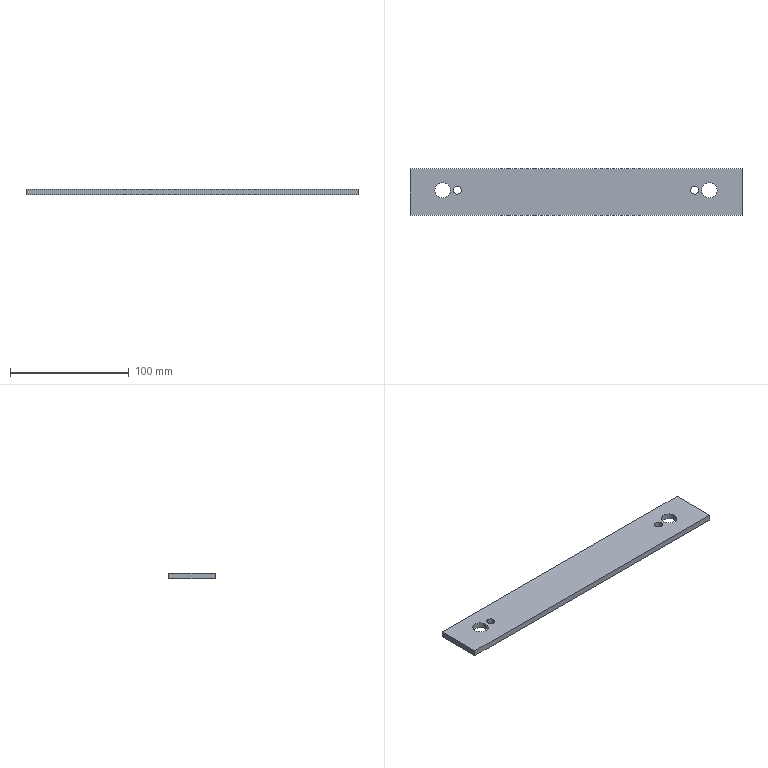Part | STEP file | 44-02-09 Ear Forming Plate B | 1 solid | 14 faces | box 280 x 39 x 5 mm | volume 52910 mm3 | cylinder 8 | plane 6 | commonest cylinder face diameters 6.8 x4 13 x4
STEP:
#1=CARTESIAN_POINT('',(0.,0.,0.));
#2=DIRECTION('',(0.,0.,1.));
#3=DIRECTION('',(1.,0.,0.));
#4=AXIS2_PLACEMENT_3D('',#1,#2,#3);
#5=CARTESIAN_POINT('',(-96.6,0.,-2.5));
#6=VERTEX_POINT('',#5);
#7=CARTESIAN_POINT('',(-96.6,0.,2.5));
#8=VERTEX_POINT('',#7);
#9=CARTESIAN_POINT('',(-96.6,0.,2.5));
#10=DIRECTION('',(0.,0.,1.));
#11=VECTOR('',#10,1.);
#12=LINE('',#9,#11);
#13=CARTESIAN_POINT('',(-100.,0.,2.5));
#14=DIRECTION('',(0.,0.,1.));
#15=DIRECTION('',(1.,0.,0.));
#16=AXIS2_PLACEMENT_3D('',#13,#14,#15);
#17=CYLINDRICAL_SURFACE('',#16,3.4);
#18=CARTESIAN_POINT('',(6.283,0.));
#19=DIRECTION('',(0.,1.));
#20=VECTOR('',#19,1.);
#21=LINE('',#18,#20);
#22=(GEOMETRIC_REPRESENTATION_CONTEXT(2)PARAMETRIC_REPRESENTATION_CONTEXT()REPRESENTATION_CONTEXT('',''));
#23=DEFINITIONAL_REPRESENTATION('',(#21),#22);
#24=PCURVE('',#17,#23);
#25=CARTESIAN_POINT('',(-100.,0.,2.5));
#26=DIRECTION('',(0.,0.,1.));
#27=DIRECTION('',(1.,0.,0.));
#28=AXIS2_PLACEMENT_3D('',#25,#26,#27);
#29=CYLINDRICAL_SURFACE('',#28,3.4);
#30=CARTESIAN_POINT('',(0.,0.));
#31=DIRECTION('',(0.,1.));
#32=VECTOR('',#31,1.);
#33=LINE('',#30,#32);
#34=(GEOMETRIC_REPRESENTATION_CONTEXT(2)PARAMETRIC_REPRESENTATION_CONTEXT()REPRESENTATION_CONTEXT('',''));
#35=DEFINITIONAL_REPRESENTATION('',(#33),#34);
#36=PCURVE('',#29,#35);
#37=SURFACE_CURVE('',#12,(#24,#36),.PCURVE_S1.);
#38=EDGE_CURVE('',#6,#8,#37,.T.);
#39=ORIENTED_EDGE('',*,*,#38,.T.);
#40=CARTESIAN_POINT('',(-103.4,0.,2.5));
#41=VERTEX_POINT('',#40);
#42=CARTESIAN_POINT('',(-100.,0.,2.5));
#43=DIRECTION('',(0.,0.,1.));
#44=DIRECTION('',(1.,0.,0.));
#45=AXIS2_PLACEMENT_3D('',#42,#43,#44);
#46=CIRCLE('',#45,3.4);
#47=CARTESIAN_POINT('',(0.,0.));
#48=DIRECTION('',(1.,0.));
#49=VECTOR('',#48,1.);
#50=LINE('',#47,#49);
#51=(GEOMETRIC_REPRESENTATION_CONTEXT(2)PARAMETRIC_REPRESENTATION_CONTEXT()REPRESENTATION_CONTEXT('',''));
#52=DEFINITIONAL_REPRESENTATION('',(#50),#51);
#53=PCURVE('',#17,#52);
#54=CARTESIAN_POINT('',(140.,-18.,2.5));
#55=DIRECTION('',(0.,0.,1.));
#56=DIRECTION('',(1.,0.,0.));
#57=AXIS2_PLACEMENT_3D('',#54,#55,#56);
#58=PLANE('',#57);
#59=CARTESIAN_POINT('',(-240.,18.));
#60=DIRECTION('',(1.,0.));
#61=AXIS2_PLACEMENT_2D('',#59,#60);
#62=CIRCLE('',#61,3.4);
#63=(GEOMETRIC_REPRESENTATION_CONTEXT(2)PARAMETRIC_REPRESENTATION_CONTEXT()REPRESENTATION_CONTEXT('',''));
#64=DEFINITIONAL_REPRESENTATION('',(#62),#63);
#65=PCURVE('',#58,#64);
#66=SURFACE_CURVE('',#46,(#53,#65),.PCURVE_S1.);
#67=EDGE_CURVE('',#41,#8,#66,.T.);
#68=ORIENTED_EDGE('',*,*,#67,.F.);
#69=CARTESIAN_POINT('',(-103.4,0.,-2.5));
#70=VERTEX_POINT('',#69);
#71=CARTESIAN_POINT('',(-103.4,0.,2.5));
#72=DIRECTION('',(0.,0.,1.));
#73=VECTOR('',#72,1.);
#74=LINE('',#71,#73);
#75=CARTESIAN_POINT('',(3.142,0.));
#76=DIRECTION('',(0.,1.));
#77=VECTOR('',#76,1.);
#78=LINE('',#75,#77);
#79=(GEOMETRIC_REPRESENTATION_CONTEXT(2)PARAMETRIC_REPRESENTATION_CONTEXT()REPRESENTATION_CONTEXT('',''));
#80=DEFINITIONAL_REPRESENTATION('',(#78),#79);
#81=PCURVE('',#17,#80);
#82=CARTESIAN_POINT('',(3.142,0.));
#83=DIRECTION('',(0.,1.));
#84=VECTOR('',#83,1.);
#85=LINE('',#82,#84);
#86=(GEOMETRIC_REPRESENTATION_CONTEXT(2)PARAMETRIC_REPRESENTATION_CONTEXT()REPRESENTATION_CONTEXT('',''));
#87=DEFINITIONAL_REPRESENTATION('',(#85),#86);
#88=PCURVE('',#29,#87);
#89=SURFACE_CURVE('',#74,(#81,#88),.PCURVE_S1.);
#90=EDGE_CURVE('',#70,#41,#89,.T.);
#91=ORIENTED_EDGE('',*,*,#90,.F.);
#92=CARTESIAN_POINT('',(-100.,0.,-2.5));
#93=DIRECTION('',(0.,0.,1.));
#94=DIRECTION('',(1.,0.,0.));
#95=AXIS2_PLACEMENT_3D('',#92,#93,#94);
#96=CIRCLE('',#95,3.4);
#97=CARTESIAN_POINT('',(0.,-5.));
#98=DIRECTION('',(1.,0.));
#99=VECTOR('',#98,1.);
#100=LINE('',#97,#99);
#101=(GEOMETRIC_REPRESENTATION_CONTEXT(2)PARAMETRIC_REPRESENTATION_CONTEXT()REPRESENTATION_CONTEXT('',''));
#102=DEFINITIONAL_REPRESENTATION('',(#100),#101);
#103=PCURVE('',#17,#102);
#104=CARTESIAN_POINT('',(140.,-18.,-2.5));
#105=DIRECTION('',(0.,0.,1.));
#106=DIRECTION('',(1.,0.,0.));
#107=AXIS2_PLACEMENT_3D('',#104,#105,#106);
#108=PLANE('',#107);
#109=CARTESIAN_POINT('',(-240.,18.));
#110=DIRECTION('',(1.,0.));
#111=AXIS2_PLACEMENT_2D('',#109,#110);
#112=CIRCLE('',#111,3.4);
#113=(GEOMETRIC_REPRESENTATION_CONTEXT(2)PARAMETRIC_REPRESENTATION_CONTEXT()REPRESENTATION_CONTEXT('',''));
#114=DEFINITIONAL_REPRESENTATION('',(#112),#113);
#115=PCURVE('',#108,#114);
#116=SURFACE_CURVE('',#96,(#103,#115),.PCURVE_S1.);
#117=EDGE_CURVE('',#70,#6,#116,.T.);
#118=ORIENTED_EDGE('',*,*,#117,.T.);
#119=EDGE_LOOP('',(#39,#68,#91,#118));
#120=FACE_BOUND('',#119,.F.);
#121=ADVANCED_FACE('',(#120),#17,.F.);
#122=CARTESIAN_POINT('',(103.4,0.,-2.5));
#123=VERTEX_POINT('',#122);
#124=CARTESIAN_POINT('',(103.4,0.,2.5));
#125=VERTEX_POINT('',#124);
#126=CARTESIAN_POINT('',(103.4,0.,2.5));
#127=DIRECTION('',(0.,0.,1.));
#128=VECTOR('',#127,1.);
#129=LINE('',#126,#128);
#130=CARTESIAN_POINT('',(100.,0.,2.5));
#131=DIRECTION('',(0.,0.,1.));
#132=DIRECTION('',(1.,0.,0.));
#133=AXIS2_PLACEMENT_3D('',#130,#131,#132);
#134=CYLINDRICAL_SURFACE('',#133,3.4);
#135=CARTESIAN_POINT('',(6.283,0.));
#136=DIRECTION('',(0.,1.));
#137=VECTOR('',#136,1.);
#138=LINE('',#135,#137);
#139=(GEOMETRIC_REPRESENTATION_CONTEXT(2)PARAMETRIC_REPRESENTATION_CONTEXT()REPRESENTATION_CONTEXT('',''));
#140=DEFINITIONAL_REPRESENTATION('',(#138),#139);
#141=PCURVE('',#134,#140);
#142=CARTESIAN_POINT('',(100.,0.,2.5));
#143=DIRECTION('',(0.,0.,1.));
#144=DIRECTION('',(1.,0.,0.));
#145=AXIS2_PLACEMENT_3D('',#142,#143,#144);
#146=CYLINDRICAL_SURFACE('',#145,3.4);
#147=CARTESIAN_POINT('',(0.,0.));
#148=DIRECTION('',(0.,1.));
#149=VECTOR('',#148,1.);
#150=LINE('',#147,#149);
#151=(GEOMETRIC_REPRESENTATION_CONTEXT(2)PARAMETRIC_REPRESENTATION_CONTEXT()REPRESENTATION_CONTEXT('',''));
#152=DEFINITIONAL_REPRESENTATION('',(#150),#151);
#153=PCURVE('',#146,#152);
#154=SURFACE_CURVE('',#129,(#141,#153),.PCURVE_S1.);
#155=EDGE_CURVE('',#123,#125,#154,.T.);
#156=ORIENTED_EDGE('',*,*,#155,.T.);
#157=CARTESIAN_POINT('',(96.6,0.,2.5));
#158=VERTEX_POINT('',#157);
#159=CARTESIAN_POINT('',(100.,0.,2.5));
#160=DIRECTION('',(0.,0.,1.));
#161=DIRECTION('',(1.,0.,0.));
#162=AXIS2_PLACEMENT_3D('',#159,#160,#161);
#163=CIRCLE('',#162,3.4);
#164=CARTESIAN_POINT('',(0.,0.));
#165=DIRECTION('',(1.,0.));
#166=VECTOR('',#165,1.);
#167=LINE('',#164,#166);
#168=(GEOMETRIC_REPRESENTATION_CONTEXT(2)PARAMETRIC_REPRESENTATION_CONTEXT()REPRESENTATION_CONTEXT('',''));
#169=DEFINITIONAL_REPRESENTATION('',(#167),#168);
#170=PCURVE('',#134,#169);
#171=CARTESIAN_POINT('',(-40.,18.));
#172=DIRECTION('',(1.,0.));
#173=AXIS2_PLACEMENT_2D('',#171,#172);
#174=CIRCLE('',#173,3.4);
#175=(GEOMETRIC_REPRESENTATION_CONTEXT(2)PARAMETRIC_REPRESENTATION_CONTEXT()REPRESENTATION_CONTEXT('',''));
#176=DEFINITIONAL_REPRESENTATION('',(#174),#175);
#177=PCURVE('',#58,#176);
#178=SURFACE_CURVE('',#163,(#170,#177),.PCURVE_S1.);
#179=EDGE_CURVE('',#158,#125,#178,.T.);
#180=ORIENTED_EDGE('',*,*,#179,.F.);
#181=CARTESIAN_POINT('',(96.6,0.,-2.5));
#182=VERTEX_POINT('',#181);
#183=CARTESIAN_POINT('',(96.6,0.,2.5));
#184=DIRECTION('',(0.,0.,1.));
#185=VECTOR('',#184,1.);
#186=LINE('',#183,#185);
#187=CARTESIAN_POINT('',(3.142,0.));
#188=DIRECTION('',(0.,1.));
#189=VECTOR('',#188,1.);
#190=LINE('',#187,#189);
#191=(GEOMETRIC_REPRESENTATION_CONTEXT(2)PARAMETRIC_REPRESENTATION_CONTEXT()REPRESENTATION_CONTEXT('',''));
#192=DEFINITIONAL_REPRESENTATION('',(#190),#191);
#193=PCURVE('',#134,#192);
#194=CARTESIAN_POINT('',(3.142,0.));
#195=DIRECTION('',(0.,1.));
#196=VECTOR('',#195,1.);
#197=LINE('',#194,#196);
#198=(GEOMETRIC_REPRESENTATION_CONTEXT(2)PARAMETRIC_REPRESENTATION_CONTEXT()REPRESENTATION_CONTEXT('',''));
#199=DEFINITIONAL_REPRESENTATION('',(#197),#198);
#200=PCURVE('',#146,#199);
#201=SURFACE_CURVE('',#186,(#193,#200),.PCURVE_S1.);
#202=EDGE_CURVE('',#182,#158,#201,.T.);
#203=ORIENTED_EDGE('',*,*,#202,.F.);
#204=CARTESIAN_POINT('',(100.,0.,-2.5));
#205=DIRECTION('',(0.,0.,1.));
#206=DIRECTION('',(1.,0.,0.));
#207=AXIS2_PLACEMENT_3D('',#204,#205,#206);
#208=CIRCLE('',#207,3.4);
#209=CARTESIAN_POINT('',(0.,-5.));
#210=DIRECTION('',(1.,0.));
#211=VECTOR('',#210,1.);
#212=LINE('',#209,#211);
#213=(GEOMETRIC_REPRESENTATION_CONTEXT(2)PARAMETRIC_REPRESENTATION_CONTEXT()REPRESENTATION_CONTEXT('',''));
#214=DEFINITIONAL_REPRESENTATION('',(#212),#213);
#215=PCURVE('',#134,#214);
#216=CARTESIAN_POINT('',(-40.,18.));
#217=DIRECTION('',(1.,0.));
#218=AXIS2_PLACEMENT_2D('',#216,#217);
#219=CIRCLE('',#218,3.4);
#220=(GEOMETRIC_REPRESENTATION_CONTEXT(2)PARAMETRIC_REPRESENTATION_CONTEXT()REPRESENTATION_CONTEXT('',''));
#221=DEFINITIONAL_REPRESENTATION('',(#219),#220);
#222=PCURVE('',#108,#221);
#223=SURFACE_CURVE('',#208,(#215,#222),.PCURVE_S1.);
#224=EDGE_CURVE('',#182,#123,#223,.T.);
#225=ORIENTED_EDGE('',*,*,#224,.T.);
#226=EDGE_LOOP('',(#156,#180,#203,#225));
#227=FACE_BOUND('',#226,.F.);
#228=ADVANCED_FACE('',(#227),#134,.F.);
#229=CARTESIAN_POINT('',(119.,0.,-2.5));
#230=VERTEX_POINT('',#229);
#231=CARTESIAN_POINT('',(119.,0.,2.5));
#232=VERTEX_POINT('',#231);
#233=CARTESIAN_POINT('',(119.,0.,-2.5));
#234=DIRECTION('',(0.,0.,1.));
#235=VECTOR('',#234,1.);
#236=LINE('',#233,#235);
#237=CARTESIAN_POINT('',(112.5,0.,-2.5));
#238=DIRECTION('',(0.,0.,1.));
#239=DIRECTION('',(1.,0.,0.));
#240=AXIS2_PLACEMENT_3D('',#237,#238,#239);
#241=CYLINDRICAL_SURFACE('',#240,6.5);
#242=CARTESIAN_POINT('',(6.283,0.));
#243=DIRECTION('',(0.,1.));
#244=VECTOR('',#243,1.);
#245=LINE('',#242,#244);
#246=(GEOMETRIC_REPRESENTATION_CONTEXT(2)PARAMETRIC_REPRESENTATION_CONTEXT()REPRESENTATION_CONTEXT('',''));
#247=DEFINITIONAL_REPRESENTATION('',(#245),#246);
#248=PCURVE('',#241,#247);
#249=CARTESIAN_POINT('',(112.5,0.,-2.5));
#250=DIRECTION('',(0.,0.,1.));
#251=DIRECTION('',(1.,0.,0.));
#252=AXIS2_PLACEMENT_3D('',#249,#250,#251);
#253=CYLINDRICAL_SURFACE('',#252,6.5);
#254=CARTESIAN_POINT('',(0.,0.));
#255=DIRECTION('',(0.,1.));
#256=VECTOR('',#255,1.);
#257=LINE('',#254,#256);
#258=(GEOMETRIC_REPRESENTATION_CONTEXT(2)PARAMETRIC_REPRESENTATION_CONTEXT()REPRESENTATION_CONTEXT('',''));
#259=DEFINITIONAL_REPRESENTATION('',(#257),#258);
#260=PCURVE('',#253,#259);
#261=SURFACE_CURVE('',#236,(#248,#260),.PCURVE_S1.);
#262=EDGE_CURVE('',#230,#232,#261,.T.);
#263=ORIENTED_EDGE('',*,*,#262,.T.);
#264=CARTESIAN_POINT('',(106.,0.,2.5));
#265=VERTEX_POINT('',#264);
#266=CARTESIAN_POINT('',(112.5,0.,2.5));
#267=DIRECTION('',(0.,0.,1.));
#268=DIRECTION('',(1.,0.,0.));
#269=AXIS2_PLACEMENT_3D('',#266,#267,#268);
#270=CIRCLE('',#269,6.5);
#271=CARTESIAN_POINT('',(0.,5.));
#272=DIRECTION('',(1.,0.));
#273=VECTOR('',#272,1.);
#274=LINE('',#271,#273);
#275=(GEOMETRIC_REPRESENTATION_CONTEXT(2)PARAMETRIC_REPRESENTATION_CONTEXT()REPRESENTATION_CONTEXT('',''));
#276=DEFINITIONAL_REPRESENTATION('',(#274),#275);
#277=PCURVE('',#241,#276);
#278=CARTESIAN_POINT('',(-27.5,18.));
#279=DIRECTION('',(1.,0.));
#280=AXIS2_PLACEMENT_2D('',#278,#279);
#281=CIRCLE('',#280,6.5);
#282=(GEOMETRIC_REPRESENTATION_CONTEXT(2)PARAMETRIC_REPRESENTATION_CONTEXT()REPRESENTATION_CONTEXT('',''));
#283=DEFINITIONAL_REPRESENTATION('',(#281),#282);
#284=PCURVE('',#58,#283);
#285=SURFACE_CURVE('',#270,(#277,#284),.PCURVE_S1.);
#286=EDGE_CURVE('',#265,#232,#285,.T.);
#287=ORIENTED_EDGE('',*,*,#286,.F.);
#288=CARTESIAN_POINT('',(106.,0.,-2.5));
#289=VERTEX_POINT('',#288);
#290=CARTESIAN_POINT('',(106.,0.,-2.5));
#291=DIRECTION('',(0.,0.,1.));
#292=VECTOR('',#291,1.);
#293=LINE('',#290,#292);
#294=CARTESIAN_POINT('',(3.142,0.));
#295=DIRECTION('',(0.,1.));
#296=VECTOR('',#295,1.);
#297=LINE('',#294,#296);
#298=(GEOMETRIC_REPRESENTATION_CONTEXT(2)PARAMETRIC_REPRESENTATION_CONTEXT()REPRESENTATION_CONTEXT('',''));
#299=DEFINITIONAL_REPRESENTATION('',(#297),#298);
#300=PCURVE('',#241,#299);
#301=CARTESIAN_POINT('',(3.142,0.));
#302=DIRECTION('',(0.,1.));
#303=VECTOR('',#302,1.);
#304=LINE('',#301,#303);
#305=(GEOMETRIC_REPRESENTATION_CONTEXT(2)PARAMETRIC_REPRESENTATION_CONTEXT()REPRESENTATION_CONTEXT('',''));
#306=DEFINITIONAL_REPRESENTATION('',(#304),#305);
#307=PCURVE('',#253,#306);
#308=SURFACE_CURVE('',#293,(#300,#307),.PCURVE_S1.);
#309=EDGE_CURVE('',#289,#265,#308,.T.);
#310=ORIENTED_EDGE('',*,*,#309,.F.);
#311=CARTESIAN_POINT('',(112.5,0.,-2.5));
#312=DIRECTION('',(0.,0.,1.));
#313=DIRECTION('',(1.,0.,0.));
#314=AXIS2_PLACEMENT_3D('',#311,#312,#313);
#315=CIRCLE('',#314,6.5);
#316=CARTESIAN_POINT('',(0.,0.));
#317=DIRECTION('',(1.,0.));
#318=VECTOR('',#317,1.);
#319=LINE('',#316,#318);
#320=(GEOMETRIC_REPRESENTATION_CONTEXT(2)PARAMETRIC_REPRESENTATION_CONTEXT()REPRESENTATION_CONTEXT('',''));
#321=DEFINITIONAL_REPRESENTATION('',(#319),#320);
#322=PCURVE('',#241,#321);
#323=CARTESIAN_POINT('',(-27.5,18.));
#324=DIRECTION('',(1.,0.));
#325=AXIS2_PLACEMENT_2D('',#323,#324);
#326=CIRCLE('',#325,6.5);
#327=(GEOMETRIC_REPRESENTATION_CONTEXT(2)PARAMETRIC_REPRESENTATION_CONTEXT()REPRESENTATION_CONTEXT('',''));
#328=DEFINITIONAL_REPRESENTATION('',(#326),#327);
#329=PCURVE('',#108,#328);
#330=SURFACE_CURVE('',#315,(#322,#329),.PCURVE_S1.);
#331=EDGE_CURVE('',#289,#230,#330,.T.);
#332=ORIENTED_EDGE('',*,*,#331,.T.);
#333=EDGE_LOOP('',(#263,#287,#310,#332));
#334=FACE_BOUND('',#333,.F.);
#335=ADVANCED_FACE('',(#334),#241,.F.);
#336=CARTESIAN_POINT('',(-106.,0.,-2.5));
#337=VERTEX_POINT('',#336);
#338=CARTESIAN_POINT('',(-106.,0.,2.5));
#339=VERTEX_POINT('',#338);
#340=CARTESIAN_POINT('',(-106.,0.,-2.5));
#341=DIRECTION('',(0.,0.,1.));
#342=VECTOR('',#341,1.);
#343=LINE('',#340,#342);
#344=CARTESIAN_POINT('',(-112.5,0.,-2.5));
#345=DIRECTION('',(0.,0.,1.));
#346=DIRECTION('',(1.,0.,0.));
#347=AXIS2_PLACEMENT_3D('',#344,#345,#346);
#348=CYLINDRICAL_SURFACE('',#347,6.5);
#349=CARTESIAN_POINT('',(6.283,0.));
#350=DIRECTION('',(0.,1.));
#351=VECTOR('',#350,1.);
#352=LINE('',#349,#351);
#353=(GEOMETRIC_REPRESENTATION_CONTEXT(2)PARAMETRIC_REPRESENTATION_CONTEXT()REPRESENTATION_CONTEXT('',''));
#354=DEFINITIONAL_REPRESENTATION('',(#352),#353);
#355=PCURVE('',#348,#354);
#356=CARTESIAN_POINT('',(-112.5,0.,-2.5));
#357=DIRECTION('',(0.,0.,1.));
#358=DIRECTION('',(1.,0.,0.));
#359=AXIS2_PLACEMENT_3D('',#356,#357,#358);
#360=CYLINDRICAL_SURFACE('',#359,6.5);
#361=CARTESIAN_POINT('',(0.,0.));
#362=DIRECTION('',(0.,1.));
#363=VECTOR('',#362,1.);
#364=LINE('',#361,#363);
#365=(GEOMETRIC_REPRESENTATION_CONTEXT(2)PARAMETRIC_REPRESENTATION_CONTEXT()REPRESENTATION_CONTEXT('',''));
#366=DEFINITIONAL_REPRESENTATION('',(#364),#365);
#367=PCURVE('',#360,#366);
#368=SURFACE_CURVE('',#343,(#355,#367),.PCURVE_S1.);
#369=EDGE_CURVE('',#337,#339,#368,.T.);
#370=ORIENTED_EDGE('',*,*,#369,.T.);
#371=CARTESIAN_POINT('',(-119.,0.,2.5));
#372=VERTEX_POINT('',#371);
#373=CARTESIAN_POINT('',(-112.5,0.,2.5));
#374=DIRECTION('',(0.,0.,1.));
#375=DIRECTION('',(1.,0.,0.));
#376=AXIS2_PLACEMENT_3D('',#373,#374,#375);
#377=CIRCLE('',#376,6.5);
#378=CARTESIAN_POINT('',(0.,5.));
#379=DIRECTION('',(1.,0.));
#380=VECTOR('',#379,1.);
#381=LINE('',#378,#380);
#382=(GEOMETRIC_REPRESENTATION_CONTEXT(2)PARAMETRIC_REPRESENTATION_CONTEXT()REPRESENTATION_CONTEXT('',''));
#383=DEFINITIONAL_REPRESENTATION('',(#381),#382);
#384=PCURVE('',#348,#383);
#385=CARTESIAN_POINT('',(-252.5,18.));
#386=DIRECTION('',(1.,0.));
#387=AXIS2_PLACEMENT_2D('',#385,#386);
#388=CIRCLE('',#387,6.5);
#389=(GEOMETRIC_REPRESENTATION_CONTEXT(2)PARAMETRIC_REPRESENTATION_CONTEXT()REPRESENTATION_CONTEXT('',''));
#390=DEFINITIONAL_REPRESENTATION('',(#388),#389);
#391=PCURVE('',#58,#390);
#392=SURFACE_CURVE('',#377,(#384,#391),.PCURVE_S1.);
#393=EDGE_CURVE('',#372,#339,#392,.T.);
#394=ORIENTED_EDGE('',*,*,#393,.F.);
#395=CARTESIAN_POINT('',(-119.,0.,-2.5));
#396=VERTEX_POINT('',#395);
#397=CARTESIAN_POINT('',(-119.,0.,-2.5));
#398=DIRECTION('',(0.,0.,1.));
#399=VECTOR('',#398,1.);
#400=LINE('',#397,#399);
#401=CARTESIAN_POINT('',(3.142,0.));
#402=DIRECTION('',(0.,1.));
#403=VECTOR('',#402,1.);
#404=LINE('',#401,#403);
#405=(GEOMETRIC_REPRESENTATION_CONTEXT(2)PARAMETRIC_REPRESENTATION_CONTEXT()REPRESENTATION_CONTEXT('',''));
#406=DEFINITIONAL_REPRESENTATION('',(#404),#405);
#407=PCURVE('',#348,#406);
#408=CARTESIAN_POINT('',(3.142,0.));
#409=DIRECTION('',(0.,1.));
#410=VECTOR('',#409,1.);
#411=LINE('',#408,#410);
#412=(GEOMETRIC_REPRESENTATION_CONTEXT(2)PARAMETRIC_REPRESENTATION_CONTEXT()REPRESENTATION_CONTEXT('',''));
#413=DEFINITIONAL_REPRESENTATION('',(#411),#412);
#414=PCURVE('',#360,#413);
#415=SURFACE_CURVE('',#400,(#407,#414),.PCURVE_S1.);
#416=EDGE_CURVE('',#396,#372,#415,.T.);
#417=ORIENTED_EDGE('',*,*,#416,.F.);
#418=CARTESIAN_POINT('',(-112.5,0.,-2.5));
#419=DIRECTION('',(0.,0.,1.));
#420=DIRECTION('',(1.,0.,0.));
#421=AXIS2_PLACEMENT_3D('',#418,#419,#420);
#422=CIRCLE('',#421,6.5);
#423=CARTESIAN_POINT('',(0.,0.));
#424=DIRECTION('',(1.,0.));
#425=VECTOR('',#424,1.);
#426=LINE('',#423,#425);
#427=(GEOMETRIC_REPRESENTATION_CONTEXT(2)PARAMETRIC_REPRESENTATION_CONTEXT()REPRESENTATION_CONTEXT('',''));
#428=DEFINITIONAL_REPRESENTATION('',(#426),#427);
#429=PCURVE('',#348,#428);
#430=CARTESIAN_POINT('',(-252.5,18.));
#431=DIRECTION('',(1.,0.));
#432=AXIS2_PLACEMENT_2D('',#430,#431);
#433=CIRCLE('',#432,6.5);
#434=(GEOMETRIC_REPRESENTATION_CONTEXT(2)PARAMETRIC_REPRESENTATION_CONTEXT()REPRESENTATION_CONTEXT('',''));
#435=DEFINITIONAL_REPRESENTATION('',(#433),#434);
#436=PCURVE('',#108,#435);
#437=SURFACE_CURVE('',#422,(#429,#436),.PCURVE_S1.);
#438=EDGE_CURVE('',#396,#337,#437,.T.);
#439=ORIENTED_EDGE('',*,*,#438,.T.);
#440=EDGE_LOOP('',(#370,#394,#417,#439));
#441=FACE_BOUND('',#440,.F.);
#442=ADVANCED_FACE('',(#441),#348,.F.);
#443=CARTESIAN_POINT('',(140.,-21.,-2.5));
#444=VERTEX_POINT('',#443);
#445=CARTESIAN_POINT('',(140.,18.,-2.5));
#446=VERTEX_POINT('',#445);
#447=CARTESIAN_POINT('',(140.,18.,-2.5));
#448=DIRECTION('',(0.,1.,0.));
#449=VECTOR('',#448,1.);
#450=LINE('',#447,#449);
#451=CARTESIAN_POINT('',(140.,18.,2.5));
#452=DIRECTION('',(-1.,0.,0.));
#453=DIRECTION('',(0.,0.,1.));
#454=AXIS2_PLACEMENT_3D('',#451,#452,#453);
#455=PLANE('',#454);
#456=CARTESIAN_POINT('',(-5.,0.));
#457=DIRECTION('',(0.,1.));
#458=VECTOR('',#457,1.);
#459=LINE('',#456,#458);
#460=(GEOMETRIC_REPRESENTATION_CONTEXT(2)PARAMETRIC_REPRESENTATION_CONTEXT()REPRESENTATION_CONTEXT('',''));
#461=DEFINITIONAL_REPRESENTATION('',(#459),#460);
#462=PCURVE('',#455,#461);
#463=CARTESIAN_POINT('',(0.,36.));
#464=DIRECTION('',(0.,1.));
#465=VECTOR('',#464,1.);
#466=LINE('',#463,#465);
#467=(GEOMETRIC_REPRESENTATION_CONTEXT(2)PARAMETRIC_REPRESENTATION_CONTEXT()REPRESENTATION_CONTEXT('',''));
#468=DEFINITIONAL_REPRESENTATION('',(#466),#467);
#469=PCURVE('',#108,#468);
#470=SURFACE_CURVE('',#450,(#462,#469),.PCURVE_S1.);
#471=EDGE_CURVE('',#444,#446,#470,.T.);
#472=ORIENTED_EDGE('',*,*,#471,.T.);
#473=CARTESIAN_POINT('',(140.,18.,2.5));
#474=VERTEX_POINT('',#473);
#475=CARTESIAN_POINT('',(140.,18.,2.5));
#476=DIRECTION('',(0.,0.,-1.));
#477=VECTOR('',#476,1.);
#478=LINE('',#475,#477);
#479=CARTESIAN_POINT('',(0.,0.));
#480=DIRECTION('',(-1.,0.));
#481=VECTOR('',#480,1.);
#482=LINE('',#479,#481);
#483=(GEOMETRIC_REPRESENTATION_CONTEXT(2)PARAMETRIC_REPRESENTATION_CONTEXT()REPRESENTATION_CONTEXT('',''));
#484=DEFINITIONAL_REPRESENTATION('',(#482),#483);
#485=PCURVE('',#455,#484);
#486=CARTESIAN_POINT('',(-140.,18.,2.5));
#487=DIRECTION('',(0.,-1.,0.));
#488=DIRECTION('',(0.,0.,-1.));
#489=AXIS2_PLACEMENT_3D('',#486,#487,#488);
#490=PLANE('',#489);
#491=CARTESIAN_POINT('',(0.,280.));
#492=DIRECTION('',(1.,0.));
#493=VECTOR('',#492,1.);
#494=LINE('',#491,#493);
#495=(GEOMETRIC_REPRESENTATION_CONTEXT(2)PARAMETRIC_REPRESENTATION_CONTEXT()REPRESENTATION_CONTEXT('',''));
#496=DEFINITIONAL_REPRESENTATION('',(#494),#495);
#497=PCURVE('',#490,#496);
#498=SURFACE_CURVE('',#478,(#485,#497),.PCURVE_S1.);
#499=EDGE_CURVE('',#474,#446,#498,.T.);
#500=ORIENTED_EDGE('',*,*,#499,.F.);
#501=CARTESIAN_POINT('',(140.,-21.,2.5));
#502=VERTEX_POINT('',#501);
#503=CARTESIAN_POINT('',(140.,18.,2.5));
#504=DIRECTION('',(0.,1.,0.));
#505=VECTOR('',#504,1.);
#506=LINE('',#503,#505);
#507=CARTESIAN_POINT('',(0.,0.));
#508=DIRECTION('',(0.,1.));
#509=VECTOR('',#508,1.);
#510=LINE('',#507,#509);
#511=(GEOMETRIC_REPRESENTATION_CONTEXT(2)PARAMETRIC_REPRESENTATION_CONTEXT()REPRESENTATION_CONTEXT('',''));
#512=DEFINITIONAL_REPRESENTATION('',(#510),#511);
#513=PCURVE('',#455,#512);
#514=CARTESIAN_POINT('',(0.,36.));
#515=DIRECTION('',(0.,1.));
#516=VECTOR('',#515,1.);
#517=LINE('',#514,#516);
#518=(GEOMETRIC_REPRESENTATION_CONTEXT(2)PARAMETRIC_REPRESENTATION_CONTEXT()REPRESENTATION_CONTEXT('',''));
#519=DEFINITIONAL_REPRESENTATION('',(#517),#518);
#520=PCURVE('',#58,#519);
#521=SURFACE_CURVE('',#506,(#513,#520),.PCURVE_S1.);
#522=EDGE_CURVE('',#502,#474,#521,.T.);
#523=ORIENTED_EDGE('',*,*,#522,.F.);
#524=CARTESIAN_POINT('',(140.,-21.,-2.5));
#525=DIRECTION('',(0.,0.,-1.));
#526=VECTOR('',#525,1.);
#527=LINE('',#524,#526);
#528=CARTESIAN_POINT('',(-5.,-39.));
#529=DIRECTION('',(-1.,0.));
#530=VECTOR('',#529,1.);
#531=LINE('',#528,#530);
#532=(GEOMETRIC_REPRESENTATION_CONTEXT(2)PARAMETRIC_REPRESENTATION_CONTEXT()REPRESENTATION_CONTEXT('',''));
#533=DEFINITIONAL_REPRESENTATION('',(#531),#532);
#534=PCURVE('',#455,#533);
#535=CARTESIAN_POINT('',(-140.,-21.,2.5));
#536=DIRECTION('',(0.,1.,0.));
#537=DIRECTION('',(0.,0.,1.));
#538=AXIS2_PLACEMENT_3D('',#535,#536,#537);
#539=PLANE('',#538);
#540=CARTESIAN_POINT('',(-5.,280.));
#541=DIRECTION('',(-1.,0.));
#542=VECTOR('',#541,1.);
#543=LINE('',#540,#542);
#544=(GEOMETRIC_REPRESENTATION_CONTEXT(2)PARAMETRIC_REPRESENTATION_CONTEXT()REPRESENTATION_CONTEXT('',''));
#545=DEFINITIONAL_REPRESENTATION('',(#543),#544);
#546=PCURVE('',#539,#545);
#547=SURFACE_CURVE('',#527,(#534,#546),.PCURVE_S1.);
#548=EDGE_CURVE('',#502,#444,#547,.T.);
#549=ORIENTED_EDGE('',*,*,#548,.T.);
#550=EDGE_LOOP('',(#472,#500,#523,#549));
#551=FACE_BOUND('',#550,.T.);
#552=ADVANCED_FACE('',(#551),#455,.F.);
#553=CARTESIAN_POINT('',(-140.,18.,-2.5));
#554=VERTEX_POINT('',#553);
#555=CARTESIAN_POINT('',(-140.,18.,-2.5));
#556=DIRECTION('',(-1.,0.,0.));
#557=VECTOR('',#556,1.);
#558=LINE('',#555,#557);
#559=CARTESIAN_POINT('',(5.,0.));
#560=DIRECTION('',(0.,-1.));
#561=VECTOR('',#560,1.);
#562=LINE('',#559,#561);
#563=(GEOMETRIC_REPRESENTATION_CONTEXT(2)PARAMETRIC_REPRESENTATION_CONTEXT()REPRESENTATION_CONTEXT('',''));
#564=DEFINITIONAL_REPRESENTATION('',(#562),#563);
#565=PCURVE('',#490,#564);
#566=CARTESIAN_POINT('',(-280.,36.));
#567=DIRECTION('',(-1.,0.));
#568=VECTOR('',#567,1.);
#569=LINE('',#566,#568);
#570=(GEOMETRIC_REPRESENTATION_CONTEXT(2)PARAMETRIC_REPRESENTATION_CONTEXT()REPRESENTATION_CONTEXT('',''));
#571=DEFINITIONAL_REPRESENTATION('',(#569),#570);
#572=PCURVE('',#108,#571);
#573=SURFACE_CURVE('',#558,(#565,#572),.PCURVE_S1.);
#574=EDGE_CURVE('',#446,#554,#573,.T.);
#575=ORIENTED_EDGE('',*,*,#574,.T.);
#576=CARTESIAN_POINT('',(-140.,18.,2.5));
#577=VERTEX_POINT('',#576);
#578=CARTESIAN_POINT('',(-140.,18.,2.5));
#579=DIRECTION('',(0.,0.,-1.));
#580=VECTOR('',#579,1.);
#581=LINE('',#578,#580);
#582=CARTESIAN_POINT('',(0.,0.));
#583=DIRECTION('',(1.,0.));
#584=VECTOR('',#583,1.);
#585=LINE('',#582,#584);
#586=(GEOMETRIC_REPRESENTATION_CONTEXT(2)PARAMETRIC_REPRESENTATION_CONTEXT()REPRESENTATION_CONTEXT('',''));
#587=DEFINITIONAL_REPRESENTATION('',(#585),#586);
#588=PCURVE('',#490,#587);
#589=CARTESIAN_POINT('',(-140.,18.,2.5));
#590=DIRECTION('',(1.,0.,0.));
#591=DIRECTION('',(0.,0.,-1.));
#592=AXIS2_PLACEMENT_3D('',#589,#590,#591);
#593=PLANE('',#592);
#594=CARTESIAN_POINT('',(0.,0.));
#595=DIRECTION('',(1.,0.));
#596=VECTOR('',#595,1.);
#597=LINE('',#594,#596);
#598=(GEOMETRIC_REPRESENTATION_CONTEXT(2)PARAMETRIC_REPRESENTATION_CONTEXT()REPRESENTATION_CONTEXT('',''));
#599=DEFINITIONAL_REPRESENTATION('',(#597),#598);
#600=PCURVE('',#593,#599);
#601=SURFACE_CURVE('',#581,(#588,#600),.PCURVE_S1.);
#602=EDGE_CURVE('',#577,#554,#601,.T.);
#603=ORIENTED_EDGE('',*,*,#602,.F.);
#604=CARTESIAN_POINT('',(-140.,18.,2.5));
#605=DIRECTION('',(-1.,0.,0.));
#606=VECTOR('',#605,1.);
#607=LINE('',#604,#606);
#608=CARTESIAN_POINT('',(0.,0.));
#609=DIRECTION('',(0.,-1.));
#610=VECTOR('',#609,1.);
#611=LINE('',#608,#610);
#612=(GEOMETRIC_REPRESENTATION_CONTEXT(2)PARAMETRIC_REPRESENTATION_CONTEXT()REPRESENTATION_CONTEXT('',''));
#613=DEFINITIONAL_REPRESENTATION('',(#611),#612);
#614=PCURVE('',#490,#613);
#615=CARTESIAN_POINT('',(-280.,36.));
#616=DIRECTION('',(-1.,0.));
#617=VECTOR('',#616,1.);
#618=LINE('',#615,#617);
#619=(GEOMETRIC_REPRESENTATION_CONTEXT(2)PARAMETRIC_REPRESENTATION_CONTEXT()REPRESENTATION_CONTEXT('',''));
#620=DEFINITIONAL_REPRESENTATION('',(#618),#619);
#621=PCURVE('',#58,#620);
#622=SURFACE_CURVE('',#607,(#614,#621),.PCURVE_S1.);
#623=EDGE_CURVE('',#474,#577,#622,.T.);
#624=ORIENTED_EDGE('',*,*,#623,.F.);
#625=ORIENTED_EDGE('',*,*,#499,.T.);
#626=EDGE_LOOP('',(#575,#603,#624,#625));
#627=FACE_BOUND('',#626,.T.);
#628=ADVANCED_FACE('',(#627),#490,.F.);
#629=CARTESIAN_POINT('',(-140.,-21.,-2.5));
#630=VERTEX_POINT('',#629);
#631=CARTESIAN_POINT('',(-140.,18.,-2.5));
#632=DIRECTION('',(0.,-1.,0.));
#633=VECTOR('',#632,1.);
#634=LINE('',#631,#633);
#635=CARTESIAN_POINT('',(5.,0.));
#636=DIRECTION('',(0.,-1.));
#637=VECTOR('',#636,1.);
#638=LINE('',#635,#637);
#639=(GEOMETRIC_REPRESENTATION_CONTEXT(2)PARAMETRIC_REPRESENTATION_CONTEXT()REPRESENTATION_CONTEXT('',''));
#640=DEFINITIONAL_REPRESENTATION('',(#638),#639);
#641=PCURVE('',#593,#640);
#642=CARTESIAN_POINT('',(-280.,36.));
#643=DIRECTION('',(0.,-1.));
#644=VECTOR('',#643,1.);
#645=LINE('',#642,#644);
#646=(GEOMETRIC_REPRESENTATION_CONTEXT(2)PARAMETRIC_REPRESENTATION_CONTEXT()REPRESENTATION_CONTEXT('',''));
#647=DEFINITIONAL_REPRESENTATION('',(#645),#646);
#648=PCURVE('',#108,#647);
#649=SURFACE_CURVE('',#634,(#641,#648),.PCURVE_S1.);
#650=EDGE_CURVE('',#554,#630,#649,.T.);
#651=ORIENTED_EDGE('',*,*,#650,.T.);
#652=CARTESIAN_POINT('',(-140.,-21.,2.5));
#653=VERTEX_POINT('',#652);
#654=CARTESIAN_POINT('',(-140.,-21.,-2.5));
#655=DIRECTION('',(0.,0.,1.));
#656=VECTOR('',#655,1.);
#657=LINE('',#654,#656);
#658=CARTESIAN_POINT('',(5.,-39.));
#659=DIRECTION('',(-1.,0.));
#660=VECTOR('',#659,1.);
#661=LINE('',#658,#660);
#662=(GEOMETRIC_REPRESENTATION_CONTEXT(2)PARAMETRIC_REPRESENTATION_CONTEXT()REPRESENTATION_CONTEXT('',''));
#663=DEFINITIONAL_REPRESENTATION('',(#661),#662);
#664=PCURVE('',#593,#663);
#665=CARTESIAN_POINT('',(-5.,0.));
#666=DIRECTION('',(1.,0.));
#667=VECTOR('',#666,1.);
#668=LINE('',#665,#667);
#669=(GEOMETRIC_REPRESENTATION_CONTEXT(2)PARAMETRIC_REPRESENTATION_CONTEXT()REPRESENTATION_CONTEXT('',''));
#670=DEFINITIONAL_REPRESENTATION('',(#668),#669);
#671=PCURVE('',#539,#670);
#672=SURFACE_CURVE('',#657,(#664,#671),.PCURVE_S1.);
#673=EDGE_CURVE('',#630,#653,#672,.T.);
#674=ORIENTED_EDGE('',*,*,#673,.T.);
#675=CARTESIAN_POINT('',(-140.,18.,2.5));
#676=DIRECTION('',(0.,-1.,0.));
#677=VECTOR('',#676,1.);
#678=LINE('',#675,#677);
#679=CARTESIAN_POINT('',(0.,0.));
#680=DIRECTION('',(0.,-1.));
#681=VECTOR('',#680,1.);
#682=LINE('',#679,#681);
#683=(GEOMETRIC_REPRESENTATION_CONTEXT(2)PARAMETRIC_REPRESENTATION_CONTEXT()REPRESENTATION_CONTEXT('',''));
#684=DEFINITIONAL_REPRESENTATION('',(#682),#683);
#685=PCURVE('',#593,#684);
#686=CARTESIAN_POINT('',(-280.,36.));
#687=DIRECTION('',(0.,-1.));
#688=VECTOR('',#687,1.);
#689=LINE('',#686,#688);
#690=(GEOMETRIC_REPRESENTATION_CONTEXT(2)PARAMETRIC_REPRESENTATION_CONTEXT()REPRESENTATION_CONTEXT('',''));
#691=DEFINITIONAL_REPRESENTATION('',(#689),#690);
#692=PCURVE('',#58,#691);
#693=SURFACE_CURVE('',#678,(#685,#692),.PCURVE_S1.);
#694=EDGE_CURVE('',#577,#653,#693,.T.);
#695=ORIENTED_EDGE('',*,*,#694,.F.);
#696=ORIENTED_EDGE('',*,*,#602,.T.);
#697=EDGE_LOOP('',(#651,#674,#695,#696));
#698=FACE_BOUND('',#697,.T.);
#699=ADVANCED_FACE('',(#698),#593,.F.);
#700=CARTESIAN_POINT('',(-100.,0.,2.5));
#701=DIRECTION('',(0.,0.,1.));
#702=DIRECTION('',(1.,0.,0.));
#703=AXIS2_PLACEMENT_3D('',#700,#701,#702);
#704=CIRCLE('',#703,3.4);
#705=CARTESIAN_POINT('',(-240.,18.));
#706=DIRECTION('',(1.,0.));
#707=AXIS2_PLACEMENT_2D('',#705,#706);
#708=CIRCLE('',#707,3.4);
#709=(GEOMETRIC_REPRESENTATION_CONTEXT(2)PARAMETRIC_REPRESENTATION_CONTEXT()REPRESENTATION_CONTEXT('',''));
#710=DEFINITIONAL_REPRESENTATION('',(#708),#709);
#711=PCURVE('',#58,#710);
#712=CARTESIAN_POINT('',(0.,0.));
#713=DIRECTION('',(1.,0.));
#714=VECTOR('',#713,1.);
#715=LINE('',#712,#714);
#716=(GEOMETRIC_REPRESENTATION_CONTEXT(2)PARAMETRIC_REPRESENTATION_CONTEXT()REPRESENTATION_CONTEXT('',''));
#717=DEFINITIONAL_REPRESENTATION('',(#715),#716);
#718=PCURVE('',#29,#717);
#719=SURFACE_CURVE('',#704,(#711,#718),.PCURVE_S1.);
#720=EDGE_CURVE('',#8,#41,#719,.T.);
#721=ORIENTED_EDGE('',*,*,#720,.F.);
#722=ORIENTED_EDGE('',*,*,#67,.F.);
#723=EDGE_LOOP('',(#721,#722));
#724=FACE_BOUND('',#723,.T.);
#725=CARTESIAN_POINT('',(100.,0.,2.5));
#726=DIRECTION('',(0.,0.,1.));
#727=DIRECTION('',(1.,0.,0.));
#728=AXIS2_PLACEMENT_3D('',#725,#726,#727);
#729=CIRCLE('',#728,3.4);
#730=CARTESIAN_POINT('',(-40.,18.));
#731=DIRECTION('',(1.,0.));
#732=AXIS2_PLACEMENT_2D('',#730,#731);
#733=CIRCLE('',#732,3.4);
#734=(GEOMETRIC_REPRESENTATION_CONTEXT(2)PARAMETRIC_REPRESENTATION_CONTEXT()REPRESENTATION_CONTEXT('',''));
#735=DEFINITIONAL_REPRESENTATION('',(#733),#734);
#736=PCURVE('',#58,#735);
#737=CARTESIAN_POINT('',(0.,0.));
#738=DIRECTION('',(1.,0.));
#739=VECTOR('',#738,1.);
#740=LINE('',#737,#739);
#741=(GEOMETRIC_REPRESENTATION_CONTEXT(2)PARAMETRIC_REPRESENTATION_CONTEXT()REPRESENTATION_CONTEXT('',''));
#742=DEFINITIONAL_REPRESENTATION('',(#740),#741);
#743=PCURVE('',#146,#742);
#744=SURFACE_CURVE('',#729,(#736,#743),.PCURVE_S1.);
#745=EDGE_CURVE('',#125,#158,#744,.T.);
#746=ORIENTED_EDGE('',*,*,#745,.F.);
#747=ORIENTED_EDGE('',*,*,#179,.F.);
#748=EDGE_LOOP('',(#746,#747));
#749=FACE_BOUND('',#748,.T.);
#750=CARTESIAN_POINT('',(112.5,0.,2.5));
#751=DIRECTION('',(0.,0.,1.));
#752=DIRECTION('',(1.,0.,0.));
#753=AXIS2_PLACEMENT_3D('',#750,#751,#752);
#754=CIRCLE('',#753,6.5);
#755=CARTESIAN_POINT('',(-27.5,18.));
#756=DIRECTION('',(1.,0.));
#757=AXIS2_PLACEMENT_2D('',#755,#756);
#758=CIRCLE('',#757,6.5);
#759=(GEOMETRIC_REPRESENTATION_CONTEXT(2)PARAMETRIC_REPRESENTATION_CONTEXT()REPRESENTATION_CONTEXT('',''));
#760=DEFINITIONAL_REPRESENTATION('',(#758),#759);
#761=PCURVE('',#58,#760);
#762=CARTESIAN_POINT('',(0.,5.));
#763=DIRECTION('',(1.,0.));
#764=VECTOR('',#763,1.);
#765=LINE('',#762,#764);
#766=(GEOMETRIC_REPRESENTATION_CONTEXT(2)PARAMETRIC_REPRESENTATION_CONTEXT()REPRESENTATION_CONTEXT('',''));
#767=DEFINITIONAL_REPRESENTATION('',(#765),#766);
#768=PCURVE('',#253,#767);
#769=SURFACE_CURVE('',#754,(#761,#768),.PCURVE_S1.);
#770=EDGE_CURVE('',#232,#265,#769,.T.);
#771=ORIENTED_EDGE('',*,*,#770,.F.);
#772=ORIENTED_EDGE('',*,*,#286,.F.);
#773=EDGE_LOOP('',(#771,#772));
#774=FACE_BOUND('',#773,.T.);
#775=CARTESIAN_POINT('',(-112.5,0.,2.5));
#776=DIRECTION('',(0.,0.,1.));
#777=DIRECTION('',(1.,0.,0.));
#778=AXIS2_PLACEMENT_3D('',#775,#776,#777);
#779=CIRCLE('',#778,6.5);
#780=CARTESIAN_POINT('',(-252.5,18.));
#781=DIRECTION('',(1.,0.));
#782=AXIS2_PLACEMENT_2D('',#780,#781);
#783=CIRCLE('',#782,6.5);
#784=(GEOMETRIC_REPRESENTATION_CONTEXT(2)PARAMETRIC_REPRESENTATION_CONTEXT()REPRESENTATION_CONTEXT('',''));
#785=DEFINITIONAL_REPRESENTATION('',(#783),#784);
#786=PCURVE('',#58,#785);
#787=CARTESIAN_POINT('',(0.,5.));
#788=DIRECTION('',(1.,0.));
#789=VECTOR('',#788,1.);
#790=LINE('',#787,#789);
#791=(GEOMETRIC_REPRESENTATION_CONTEXT(2)PARAMETRIC_REPRESENTATION_CONTEXT()REPRESENTATION_CONTEXT('',''));
#792=DEFINITIONAL_REPRESENTATION('',(#790),#791);
#793=PCURVE('',#360,#792);
#794=SURFACE_CURVE('',#779,(#786,#793),.PCURVE_S1.);
#795=EDGE_CURVE('',#339,#372,#794,.T.);
#796=ORIENTED_EDGE('',*,*,#795,.F.);
#797=ORIENTED_EDGE('',*,*,#393,.F.);
#798=EDGE_LOOP('',(#796,#797));
#799=FACE_BOUND('',#798,.T.);
#800=ORIENTED_EDGE('',*,*,#522,.T.);
#801=ORIENTED_EDGE('',*,*,#623,.T.);
#802=ORIENTED_EDGE('',*,*,#694,.T.);
#803=CARTESIAN_POINT('',(-140.,-21.,2.5));
#804=DIRECTION('',(1.,0.,0.));
#805=VECTOR('',#804,1.);
#806=LINE('',#803,#805);
#807=CARTESIAN_POINT('',(-280.,-3.));
#808=DIRECTION('',(1.,0.));
#809=VECTOR('',#808,1.);
#810=LINE('',#807,#809);
#811=(GEOMETRIC_REPRESENTATION_CONTEXT(2)PARAMETRIC_REPRESENTATION_CONTEXT()REPRESENTATION_CONTEXT('',''));
#812=DEFINITIONAL_REPRESENTATION('',(#810),#811);
#813=PCURVE('',#58,#812);
#814=CARTESIAN_POINT('',(0.,0.));
#815=DIRECTION('',(0.,1.));
#816=VECTOR('',#815,1.);
#817=LINE('',#814,#816);
#818=(GEOMETRIC_REPRESENTATION_CONTEXT(2)PARAMETRIC_REPRESENTATION_CONTEXT()REPRESENTATION_CONTEXT('',''));
#819=DEFINITIONAL_REPRESENTATION('',(#817),#818);
#820=PCURVE('',#539,#819);
#821=SURFACE_CURVE('',#806,(#813,#820),.PCURVE_S1.);
#822=EDGE_CURVE('',#653,#502,#821,.T.);
#823=ORIENTED_EDGE('',*,*,#822,.T.);
#824=EDGE_LOOP('',(#800,#801,#802,#823));
#825=FACE_BOUND('',#824,.T.);
#826=ADVANCED_FACE('',(#724,#749,#774,#799,#825),#58,.T.);
#827=CARTESIAN_POINT('',(-100.,0.,-2.5));
#828=DIRECTION('',(0.,0.,1.));
#829=DIRECTION('',(1.,0.,0.));
#830=AXIS2_PLACEMENT_3D('',#827,#828,#829);
#831=CIRCLE('',#830,3.4);
#832=CARTESIAN_POINT('',(-240.,18.));
#833=DIRECTION('',(1.,0.));
#834=AXIS2_PLACEMENT_2D('',#832,#833);
#835=CIRCLE('',#834,3.4);
#836=(GEOMETRIC_REPRESENTATION_CONTEXT(2)PARAMETRIC_REPRESENTATION_CONTEXT()REPRESENTATION_CONTEXT('',''));
#837=DEFINITIONAL_REPRESENTATION('',(#835),#836);
#838=PCURVE('',#108,#837);
#839=CARTESIAN_POINT('',(0.,-5.));
#840=DIRECTION('',(1.,0.));
#841=VECTOR('',#840,1.);
#842=LINE('',#839,#841);
#843=(GEOMETRIC_REPRESENTATION_CONTEXT(2)PARAMETRIC_REPRESENTATION_CONTEXT()REPRESENTATION_CONTEXT('',''));
#844=DEFINITIONAL_REPRESENTATION('',(#842),#843);
#845=PCURVE('',#29,#844);
#846=SURFACE_CURVE('',#831,(#838,#845),.PCURVE_S1.);
#847=EDGE_CURVE('',#6,#70,#846,.T.);
#848=ORIENTED_EDGE('',*,*,#847,.T.);
#849=ORIENTED_EDGE('',*,*,#117,.T.);
#850=EDGE_LOOP('',(#848,#849));
#851=FACE_BOUND('',#850,.T.);
#852=CARTESIAN_POINT('',(100.,0.,-2.5));
#853=DIRECTION('',(0.,0.,1.));
#854=DIRECTION('',(1.,0.,0.));
#855=AXIS2_PLACEMENT_3D('',#852,#853,#854);
#856=CIRCLE('',#855,3.4);
#857=CARTESIAN_POINT('',(-40.,18.));
#858=DIRECTION('',(1.,0.));
#859=AXIS2_PLACEMENT_2D('',#857,#858);
#860=CIRCLE('',#859,3.4);
#861=(GEOMETRIC_REPRESENTATION_CONTEXT(2)PARAMETRIC_REPRESENTATION_CONTEXT()REPRESENTATION_CONTEXT('',''));
#862=DEFINITIONAL_REPRESENTATION('',(#860),#861);
#863=PCURVE('',#108,#862);
#864=CARTESIAN_POINT('',(0.,-5.));
#865=DIRECTION('',(1.,0.));
#866=VECTOR('',#865,1.);
#867=LINE('',#864,#866);
#868=(GEOMETRIC_REPRESENTATION_CONTEXT(2)PARAMETRIC_REPRESENTATION_CONTEXT()REPRESENTATION_CONTEXT('',''));
#869=DEFINITIONAL_REPRESENTATION('',(#867),#868);
#870=PCURVE('',#146,#869);
#871=SURFACE_CURVE('',#856,(#863,#870),.PCURVE_S1.);
#872=EDGE_CURVE('',#123,#182,#871,.T.);
#873=ORIENTED_EDGE('',*,*,#872,.T.);
#874=ORIENTED_EDGE('',*,*,#224,.T.);
#875=EDGE_LOOP('',(#873,#874));
#876=FACE_BOUND('',#875,.T.);
#877=CARTESIAN_POINT('',(112.5,0.,-2.5));
#878=DIRECTION('',(0.,0.,1.));
#879=DIRECTION('',(1.,0.,0.));
#880=AXIS2_PLACEMENT_3D('',#877,#878,#879);
#881=CIRCLE('',#880,6.5);
#882=CARTESIAN_POINT('',(-27.5,18.));
#883=DIRECTION('',(1.,0.));
#884=AXIS2_PLACEMENT_2D('',#882,#883);
#885=CIRCLE('',#884,6.5);
#886=(GEOMETRIC_REPRESENTATION_CONTEXT(2)PARAMETRIC_REPRESENTATION_CONTEXT()REPRESENTATION_CONTEXT('',''));
#887=DEFINITIONAL_REPRESENTATION('',(#885),#886);
#888=PCURVE('',#108,#887);
#889=CARTESIAN_POINT('',(0.,0.));
#890=DIRECTION('',(1.,0.));
#891=VECTOR('',#890,1.);
#892=LINE('',#889,#891);
#893=(GEOMETRIC_REPRESENTATION_CONTEXT(2)PARAMETRIC_REPRESENTATION_CONTEXT()REPRESENTATION_CONTEXT('',''));
#894=DEFINITIONAL_REPRESENTATION('',(#892),#893);
#895=PCURVE('',#253,#894);
#896=SURFACE_CURVE('',#881,(#888,#895),.PCURVE_S1.);
#897=EDGE_CURVE('',#230,#289,#896,.T.);
#898=ORIENTED_EDGE('',*,*,#897,.T.);
#899=ORIENTED_EDGE('',*,*,#331,.T.);
#900=EDGE_LOOP('',(#898,#899));
#901=FACE_BOUND('',#900,.T.);
#902=CARTESIAN_POINT('',(-112.5,0.,-2.5));
#903=DIRECTION('',(0.,0.,1.));
#904=DIRECTION('',(1.,0.,0.));
#905=AXIS2_PLACEMENT_3D('',#902,#903,#904);
#906=CIRCLE('',#905,6.5);
#907=CARTESIAN_POINT('',(-252.5,18.));
#908=DIRECTION('',(1.,0.));
#909=AXIS2_PLACEMENT_2D('',#907,#908);
#910=CIRCLE('',#909,6.5);
#911=(GEOMETRIC_REPRESENTATION_CONTEXT(2)PARAMETRIC_REPRESENTATION_CONTEXT()REPRESENTATION_CONTEXT('',''));
#912=DEFINITIONAL_REPRESENTATION('',(#910),#911);
#913=PCURVE('',#108,#912);
#914=CARTESIAN_POINT('',(0.,0.));
#915=DIRECTION('',(1.,0.));
#916=VECTOR('',#915,1.);
#917=LINE('',#914,#916);
#918=(GEOMETRIC_REPRESENTATION_CONTEXT(2)PARAMETRIC_REPRESENTATION_CONTEXT()REPRESENTATION_CONTEXT('',''));
#919=DEFINITIONAL_REPRESENTATION('',(#917),#918);
#920=PCURVE('',#360,#919);
#921=SURFACE_CURVE('',#906,(#913,#920),.PCURVE_S1.);
#922=EDGE_CURVE('',#337,#396,#921,.T.);
#923=ORIENTED_EDGE('',*,*,#922,.T.);
#924=ORIENTED_EDGE('',*,*,#438,.T.);
#925=EDGE_LOOP('',(#923,#924));
#926=FACE_BOUND('',#925,.T.);
#927=ORIENTED_EDGE('',*,*,#471,.F.);
#928=CARTESIAN_POINT('',(-140.,-21.,-2.5));
#929=DIRECTION('',(-1.,0.,0.));
#930=VECTOR('',#929,1.);
#931=LINE('',#928,#930);
#932=CARTESIAN_POINT('',(-280.,-3.));
#933=DIRECTION('',(-1.,0.));
#934=VECTOR('',#933,1.);
#935=LINE('',#932,#934);
#936=(GEOMETRIC_REPRESENTATION_CONTEXT(2)PARAMETRIC_REPRESENTATION_CONTEXT()REPRESENTATION_CONTEXT('',''));
#937=DEFINITIONAL_REPRESENTATION('',(#935),#936);
#938=PCURVE('',#108,#937);
#939=CARTESIAN_POINT('',(-5.,0.));
#940=DIRECTION('',(0.,-1.));
#941=VECTOR('',#940,1.);
#942=LINE('',#939,#941);
#943=(GEOMETRIC_REPRESENTATION_CONTEXT(2)PARAMETRIC_REPRESENTATION_CONTEXT()REPRESENTATION_CONTEXT('',''));
#944=DEFINITIONAL_REPRESENTATION('',(#942),#943);
#945=PCURVE('',#539,#944);
#946=SURFACE_CURVE('',#931,(#938,#945),.PCURVE_S1.);
#947=EDGE_CURVE('',#444,#630,#946,.T.);
#948=ORIENTED_EDGE('',*,*,#947,.T.);
#949=ORIENTED_EDGE('',*,*,#650,.F.);
#950=ORIENTED_EDGE('',*,*,#574,.F.);
#951=EDGE_LOOP('',(#927,#948,#949,#950));
#952=FACE_BOUND('',#951,.T.);
#953=ADVANCED_FACE('',(#851,#876,#901,#926,#952),#108,.F.);
#954=ORIENTED_EDGE('',*,*,#795,.F.);
#955=ORIENTED_EDGE('',*,*,#369,.F.);
#956=ORIENTED_EDGE('',*,*,#922,.T.);
#957=ORIENTED_EDGE('',*,*,#416,.T.);
#958=EDGE_LOOP('',(#954,#955,#956,#957));
#959=FACE_BOUND('',#958,.F.);
#960=ADVANCED_FACE('',(#959),#360,.F.);
#961=ORIENTED_EDGE('',*,*,#770,.F.);
#962=ORIENTED_EDGE('',*,*,#262,.F.);
#963=ORIENTED_EDGE('',*,*,#897,.T.);
#964=ORIENTED_EDGE('',*,*,#309,.T.);
#965=EDGE_LOOP('',(#961,#962,#963,#964));
#966=FACE_BOUND('',#965,.F.);
#967=ADVANCED_FACE('',(#966),#253,.F.);
#968=ORIENTED_EDGE('',*,*,#745,.F.);
#969=ORIENTED_EDGE('',*,*,#155,.F.);
#970=ORIENTED_EDGE('',*,*,#872,.T.);
#971=ORIENTED_EDGE('',*,*,#202,.T.);
#972=EDGE_LOOP('',(#968,#969,#970,#971));
#973=FACE_BOUND('',#972,.F.);
#974=ADVANCED_FACE('',(#973),#146,.F.);
#975=ORIENTED_EDGE('',*,*,#720,.F.);
#976=ORIENTED_EDGE('',*,*,#38,.F.);
#977=ORIENTED_EDGE('',*,*,#847,.T.);
#978=ORIENTED_EDGE('',*,*,#90,.T.);
#979=EDGE_LOOP('',(#975,#976,#977,#978));
#980=FACE_BOUND('',#979,.F.);
#981=ADVANCED_FACE('',(#980),#29,.F.);
#982=ORIENTED_EDGE('',*,*,#673,.F.);
#983=ORIENTED_EDGE('',*,*,#947,.F.);
#984=ORIENTED_EDGE('',*,*,#548,.F.);
#985=ORIENTED_EDGE('',*,*,#822,.F.);
#986=EDGE_LOOP('',(#982,#983,#984,#985));
#987=FACE_BOUND('',#986,.T.);
#988=ADVANCED_FACE('',(#987),#539,.F.);
#989=CLOSED_SHELL('',(#121,#228,#335,#442,#552,#628,#699,#826,#953,#960,#967,#974,#981,#988));
#990=MANIFOLD_SOLID_BREP('',#989);
#991=(LENGTH_UNIT()NAMED_UNIT(*)SI_UNIT(.MILLI.,.METRE.));
#992=UNCERTAINTY_MEASURE_WITH_UNIT(LENGTH_MEASURE(0.0000001),#991,'','');
#993=(NAMED_UNIT(*)PLANE_ANGLE_UNIT()SI_UNIT($,.RADIAN.));
#994=(NAMED_UNIT(*)SI_UNIT($,.STERADIAN.)SOLID_ANGLE_UNIT());
#995=(GEOMETRIC_REPRESENTATION_CONTEXT(3)GLOBAL_UNCERTAINTY_ASSIGNED_CONTEXT((#992))GLOBAL_UNIT_ASSIGNED_CONTEXT((#991,#993,#994))REPRESENTATION_CONTEXT('',''));
#996=ADVANCED_BREP_SHAPE_REPRESENTATION('',(#4,#990),#995);